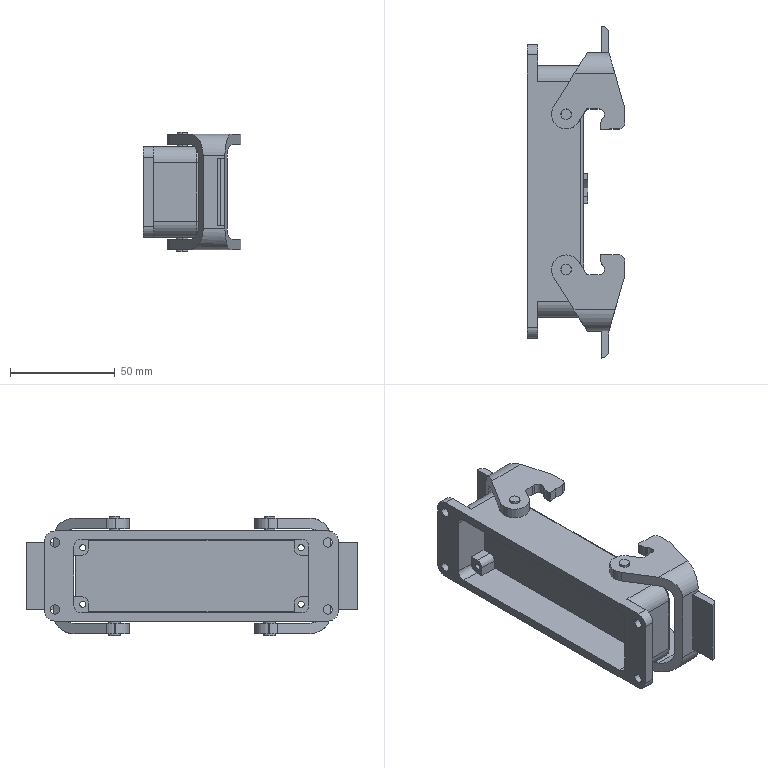Part | STEP file | 4-20.sldasm-Part-1 | 1 solid | 274 faces | box 46.6 x 158.128 x 57 mm | volume 97175 mm3 | plane 140 | cylinder 126 | torus 8 | commonest cylinder face diameters 2 x20 7 x12 3 x8 3.3 x8 4.4 x8 5.5 x8